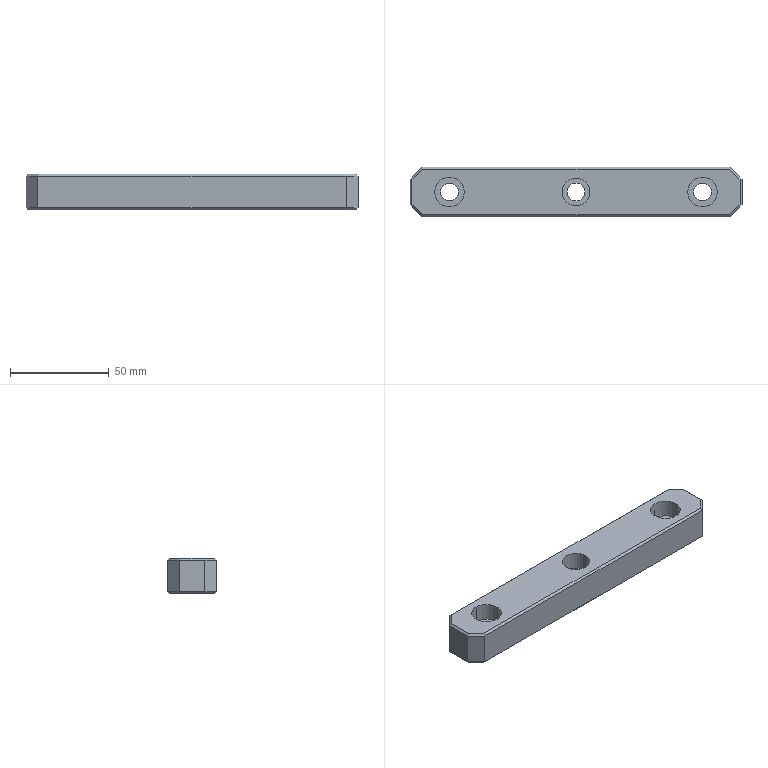Part | Creo | 1 solid | 41 faces | box 168 x 25 x 18 mm | volume 67650 mm3 | plane 29 | cylinder 12 | commonest cylinder face diameters 9 x6 15 x4 14 x2
STEP:
#1=CARTESIAN_POINT('',(281.586,11.495,-63.491));
#2=VERTEX_POINT('',#1);
#3=CARTESIAN_POINT('',(287.,6.081,-63.491));
#4=VERTEX_POINT('',#3);
#5=CARTESIAN_POINT('',(281.586,11.495,-63.491));
#6=DIRECTION('',(0.7071,-0.7071,0.));
#7=VECTOR('',#6,7.657);
#8=LINE('',#5,#7);
#9=EDGE_CURVE('',#2,#4,#8,.T.);
#10=ORIENTED_EDGE('',*,*,#9,.F.);
#11=CARTESIAN_POINT('',(126.414,11.495,-63.491));
#12=VERTEX_POINT('',#11);
#13=CARTESIAN_POINT('',(126.414,11.495,-63.491));
#14=DIRECTION('',(1.,0.,0.));
#15=VECTOR('',#14,155.172);
#16=LINE('',#13,#15);
#17=EDGE_CURVE('',#12,#2,#16,.T.);
#18=ORIENTED_EDGE('',*,*,#17,.F.);
#19=CARTESIAN_POINT('',(121.,6.081,-63.491));
#20=VERTEX_POINT('',#19);
#21=CARTESIAN_POINT('',(121.,6.081,-63.491));
#22=DIRECTION('',(0.7071,0.7071,0.));
#23=VECTOR('',#22,7.657);
#24=LINE('',#21,#23);
#25=EDGE_CURVE('',#20,#12,#24,.T.);
#26=ORIENTED_EDGE('',*,*,#25,.F.);
#27=CARTESIAN_POINT('',(121.,-6.09,-63.491));
#28=VERTEX_POINT('',#27);
#29=CARTESIAN_POINT('',(121.,-6.09,-63.491));
#30=DIRECTION('',(0.,1.,0.));
#31=VECTOR('',#30,12.172);
#32=LINE('',#29,#31);
#33=EDGE_CURVE('',#28,#20,#32,.T.);
#34=ORIENTED_EDGE('',*,*,#33,.F.);
#35=CARTESIAN_POINT('',(126.414,-11.505,-63.491));
#36=VERTEX_POINT('',#35);
#37=CARTESIAN_POINT('',(126.414,-11.505,-63.491));
#38=DIRECTION('',(-0.7071,0.7071,0.));
#39=VECTOR('',#38,7.657);
#40=LINE('',#37,#39);
#41=EDGE_CURVE('',#36,#28,#40,.T.);
#42=ORIENTED_EDGE('',*,*,#41,.F.);
#43=CARTESIAN_POINT('',(281.586,-11.505,-63.491));
#44=VERTEX_POINT('',#43);
#45=CARTESIAN_POINT('',(126.414,-11.505,-63.491));
#46=DIRECTION('',(1.,0.,0.));
#47=VECTOR('',#46,155.172);
#48=LINE('',#45,#47);
#49=EDGE_CURVE('',#36,#44,#48,.T.);
#50=ORIENTED_EDGE('',*,*,#49,.T.);
#51=CARTESIAN_POINT('',(287.,-6.09,-63.491));
#52=VERTEX_POINT('',#51);
#53=CARTESIAN_POINT('',(287.,-6.09,-63.491));
#54=DIRECTION('',(-0.7071,-0.7071,0.));
#55=VECTOR('',#54,7.657);
#56=LINE('',#53,#55);
#57=EDGE_CURVE('',#52,#44,#56,.T.);
#58=ORIENTED_EDGE('',*,*,#57,.F.);
#59=CARTESIAN_POINT('',(287.,6.081,-63.491));
#60=DIRECTION('',(0.,-1.,0.));
#61=VECTOR('',#60,12.172);
#62=LINE('',#59,#61);
#63=EDGE_CURVE('',#4,#52,#62,.T.);
#64=ORIENTED_EDGE('',*,*,#63,.F.);
#65=EDGE_LOOP('',(#10,#18,#26,#34,#42,#50,#58,#64));
#66=FACE_OUTER_BOUND('',#65,.F.);
#67=CARTESIAN_POINT('',(140.,-4.505,-63.491));
#68=VERTEX_POINT('',#67);
#69=CARTESIAN_POINT('',(140.,4.495,-63.491));
#70=VERTEX_POINT('',#69);
#71=CARTESIAN_POINT('',(140.,-0.004699,-63.491));
#72=DIRECTION('',(0.,0.,1.));
#73=DIRECTION('',(0.,-1.,0.));
#74=AXIS2_PLACEMENT_3D('',#71,#72,#73);
#75=CIRCLE('',#74,4.5);
#76=EDGE_CURVE('',#68,#70,#75,.T.);
#77=ORIENTED_EDGE('',*,*,#76,.F.);
#78=CARTESIAN_POINT('',(140.,-0.004699,-63.491));
#79=DIRECTION('',(0.,0.,1.));
#80=DIRECTION('',(0.,1.,0.));
#81=AXIS2_PLACEMENT_3D('',#78,#79,#80);
#82=CIRCLE('',#81,4.5);
#83=EDGE_CURVE('',#70,#68,#82,.T.);
#84=ORIENTED_EDGE('',*,*,#83,.F.);
#85=EDGE_LOOP('',(#77,#84));
#86=FACE_BOUND('',#85,.F.);
#87=CARTESIAN_POINT('',(268.,-4.505,-63.491));
#88=VERTEX_POINT('',#87);
#89=CARTESIAN_POINT('',(268.,4.495,-63.491));
#90=VERTEX_POINT('',#89);
#91=CARTESIAN_POINT('',(268.,-0.004699,-63.491));
#92=DIRECTION('',(0.,0.,1.));
#93=DIRECTION('',(0.,-1.,0.));
#94=AXIS2_PLACEMENT_3D('',#91,#92,#93);
#95=CIRCLE('',#94,4.5);
#96=EDGE_CURVE('',#88,#90,#95,.T.);
#97=ORIENTED_EDGE('',*,*,#96,.F.);
#98=CARTESIAN_POINT('',(268.,-0.004699,-63.491));
#99=DIRECTION('',(0.,0.,1.));
#100=DIRECTION('',(0.,1.,0.));
#101=AXIS2_PLACEMENT_3D('',#98,#99,#100);
#102=CIRCLE('',#101,4.5);
#103=EDGE_CURVE('',#90,#88,#102,.T.);
#104=ORIENTED_EDGE('',*,*,#103,.F.);
#105=EDGE_LOOP('',(#97,#104));
#106=FACE_BOUND('',#105,.F.);
#107=CARTESIAN_POINT('',(208.5,-0.004699,-63.491));
#108=VERTEX_POINT('',#107);
#109=CARTESIAN_POINT('',(199.5,-0.004699,-63.491));
#110=VERTEX_POINT('',#109);
#111=CARTESIAN_POINT('',(204.,-0.004699,-63.491));
#112=DIRECTION('',(0.,0.,1.));
#113=DIRECTION('',(1.,0.,0.));
#114=AXIS2_PLACEMENT_3D('',#111,#112,#113);
#115=CIRCLE('',#114,4.5);
#116=EDGE_CURVE('',#108,#110,#115,.T.);
#117=ORIENTED_EDGE('',*,*,#116,.F.);
#118=CARTESIAN_POINT('',(204.,-0.004699,-63.491));
#119=DIRECTION('',(0.,0.,1.));
#120=DIRECTION('',(-1.,0.,0.));
#121=AXIS2_PLACEMENT_3D('',#118,#119,#120);
#122=CIRCLE('',#121,4.5);
#123=EDGE_CURVE('',#110,#108,#122,.T.);
#124=ORIENTED_EDGE('',*,*,#123,.F.);
#125=EDGE_LOOP('',(#117,#124));
#126=FACE_BOUND('',#125,.F.);
#127=CARTESIAN_POINT('',(270.,-12.505,-63.491));
#128=DIRECTION('',(0.,0.,-1.));
#129=DIRECTION('',(0.,1.,0.));
#130=AXIS2_PLACEMENT_3D('',#127,#128,#129);
#131=PLANE('',#130);
#132=ADVANCED_FACE('',(#66,#86,#106,#126),#131,.T.);
#133=ORIENTED_EDGE('',*,*,#9,.T.);
#134=CARTESIAN_POINT('',(288.,6.495,-62.491));
#135=VERTEX_POINT('',#134);
#136=CARTESIAN_POINT('',(287.,6.081,-63.491));
#137=DIRECTION('',(0.6786,0.2811,0.6786));
#138=VECTOR('',#137,1.474);
#139=LINE('',#136,#138);
#140=EDGE_CURVE('',#4,#135,#139,.T.);
#141=ORIENTED_EDGE('',*,*,#140,.T.);
#142=CARTESIAN_POINT('',(282.,12.495,-62.491));
#143=VERTEX_POINT('',#142);
#144=CARTESIAN_POINT('',(288.,6.495,-62.491));
#145=DIRECTION('',(-0.7071,0.7071,0.));
#146=VECTOR('',#145,8.485);
#147=LINE('',#144,#146);
#148=EDGE_CURVE('',#135,#143,#147,.T.);
#149=ORIENTED_EDGE('',*,*,#148,.T.);
#150=CARTESIAN_POINT('',(281.586,11.495,-63.491));
#151=DIRECTION('',(0.2811,0.6786,0.6786));
#152=VECTOR('',#151,1.474);
#153=LINE('',#150,#152);
#154=EDGE_CURVE('',#2,#143,#153,.T.);
#155=ORIENTED_EDGE('',*,*,#154,.F.);
#156=EDGE_LOOP('',(#133,#141,#149,#155));
#157=FACE_OUTER_BOUND('',#156,.F.);
#158=CARTESIAN_POINT('',(284.646,9.142,-62.991));
#159=DIRECTION('',(0.5,0.5,-0.7071));
#160=DIRECTION('',(0.5,0.5,0.7071));
#161=AXIS2_PLACEMENT_3D('',#158,#159,#160);
#162=PLANE('',#161);
#163=ADVANCED_FACE('',(#157),#162,.T.);
#164=ORIENTED_EDGE('',*,*,#63,.T.);
#165=CARTESIAN_POINT('',(288.,-6.505,-62.491));
#166=VERTEX_POINT('',#165);
#167=CARTESIAN_POINT('',(287.,-6.09,-63.491));
#168=DIRECTION('',(0.6786,-0.2811,0.6786));
#169=VECTOR('',#168,1.474);
#170=LINE('',#167,#169);
#171=EDGE_CURVE('',#52,#166,#170,.T.);
#172=ORIENTED_EDGE('',*,*,#171,.T.);
#173=CARTESIAN_POINT('',(288.,6.495,-62.491));
#174=DIRECTION('',(0.,-1.,0.));
#175=VECTOR('',#174,13.);
#176=LINE('',#173,#175);
#177=EDGE_CURVE('',#135,#166,#176,.T.);
#178=ORIENTED_EDGE('',*,*,#177,.F.);
#179=ORIENTED_EDGE('',*,*,#140,.F.);
#180=EDGE_LOOP('',(#164,#172,#178,#179));
#181=FACE_OUTER_BOUND('',#180,.F.);
#182=CARTESIAN_POINT('',(287.5,-0.004699,-62.991));
#183=DIRECTION('',(0.7071,0.,-0.7071));
#184=DIRECTION('',(-0.7071,0.,-0.7071));
#185=AXIS2_PLACEMENT_3D('',#182,#183,#184);
#186=PLANE('',#185);
#187=ADVANCED_FACE('',(#181),#186,.T.);
#188=ORIENTED_EDGE('',*,*,#57,.T.);
#189=CARTESIAN_POINT('',(282.,-12.505,-62.491));
#190=VERTEX_POINT('',#189);
#191=CARTESIAN_POINT('',(281.586,-11.505,-63.491));
#192=DIRECTION('',(0.2811,-0.6786,0.6786));
#193=VECTOR('',#192,1.474);
#194=LINE('',#191,#193);
#195=EDGE_CURVE('',#44,#190,#194,.T.);
#196=ORIENTED_EDGE('',*,*,#195,.T.);
#197=CARTESIAN_POINT('',(282.,-12.505,-62.491));
#198=DIRECTION('',(0.7071,0.7071,0.));
#199=VECTOR('',#198,8.485);
#200=LINE('',#197,#199);
#201=EDGE_CURVE('',#190,#166,#200,.T.);
#202=ORIENTED_EDGE('',*,*,#201,.T.);
#203=ORIENTED_EDGE('',*,*,#171,.F.);
#204=EDGE_LOOP('',(#188,#196,#202,#203));
#205=FACE_OUTER_BOUND('',#204,.F.);
#206=CARTESIAN_POINT('',(284.646,-9.151,-62.991));
#207=DIRECTION('',(0.5,-0.5,-0.7071));
#208=DIRECTION('',(0.5,-0.5,0.7071));
#209=AXIS2_PLACEMENT_3D('',#206,#207,#208);
#210=PLANE('',#209);
#211=ADVANCED_FACE('',(#205),#210,.T.);
#212=CARTESIAN_POINT('',(126.,-12.505,-62.491));
#213=VERTEX_POINT('',#212);
#214=CARTESIAN_POINT('',(126.,-12.505,-62.491));
#215=DIRECTION('',(0.2811,0.6786,-0.6786));
#216=VECTOR('',#215,1.474);
#217=LINE('',#214,#216);
#218=EDGE_CURVE('',#213,#36,#217,.T.);
#219=ORIENTED_EDGE('',*,*,#218,.F.);
#220=CARTESIAN_POINT('',(126.,-12.505,-62.491));
#221=DIRECTION('',(1.,0.,0.));
#222=VECTOR('',#221,156.);
#223=LINE('',#220,#222);
#224=EDGE_CURVE('',#213,#190,#223,.T.);
#225=ORIENTED_EDGE('',*,*,#224,.T.);
#226=ORIENTED_EDGE('',*,*,#195,.F.);
#227=ORIENTED_EDGE('',*,*,#49,.F.);
#228=EDGE_LOOP('',(#219,#225,#226,#227));
#229=FACE_OUTER_BOUND('',#228,.F.);
#230=CARTESIAN_POINT('',(174.,-12.005,-62.991));
#231=DIRECTION('',(0.,-0.7071,-0.7071));
#232=DIRECTION('',(0.,-0.7071,0.7071));
#233=AXIS2_PLACEMENT_3D('',#230,#231,#232);
#234=PLANE('',#233);
#235=ADVANCED_FACE('',(#229),#234,.T.);
#236=CARTESIAN_POINT('',(120.,-6.505,-62.491));
#237=VERTEX_POINT('',#236);
#238=CARTESIAN_POINT('',(120.,-6.505,-62.491));
#239=DIRECTION('',(0.7071,-0.7071,0.));
#240=VECTOR('',#239,8.485);
#241=LINE('',#238,#240);
#242=EDGE_CURVE('',#237,#213,#241,.T.);
#243=ORIENTED_EDGE('',*,*,#242,.T.);
#244=ORIENTED_EDGE('',*,*,#218,.T.);
#245=ORIENTED_EDGE('',*,*,#41,.T.);
#246=CARTESIAN_POINT('',(121.,-6.09,-63.491));
#247=DIRECTION('',(-0.6786,-0.2811,0.6786));
#248=VECTOR('',#247,1.474);
#249=LINE('',#246,#248);
#250=EDGE_CURVE('',#28,#237,#249,.T.);
#251=ORIENTED_EDGE('',*,*,#250,.T.);
#252=EDGE_LOOP('',(#243,#244,#245,#251));
#253=FACE_OUTER_BOUND('',#252,.F.);
#254=CARTESIAN_POINT('',(123.354,-9.151,-62.991));
#255=DIRECTION('',(-0.5,-0.5,-0.7071));
#256=DIRECTION('',(-0.5,-0.5,0.7071));
#257=AXIS2_PLACEMENT_3D('',#254,#255,#256);
#258=PLANE('',#257);
#259=ADVANCED_FACE('',(#253),#258,.T.);
#260=CARTESIAN_POINT('',(126.,-12.505,-46.491));
#261=VERTEX_POINT('',#260);
#262=CARTESIAN_POINT('',(126.,-12.505,-46.491));
#263=DIRECTION('',(0.,0.,-1.));
#264=VECTOR('',#263,16.);
#265=LINE('',#262,#264);
#266=EDGE_CURVE('',#261,#213,#265,.T.);
#267=ORIENTED_EDGE('',*,*,#266,.T.);
#268=ORIENTED_EDGE('',*,*,#242,.F.);
#269=CARTESIAN_POINT('',(120.,-6.505,-46.491));
#270=VERTEX_POINT('',#269);
#271=CARTESIAN_POINT('',(120.,-6.505,-46.491));
#272=DIRECTION('',(0.,0.,-1.));
#273=VECTOR('',#272,16.);
#274=LINE('',#271,#273);
#275=EDGE_CURVE('',#270,#237,#274,.T.);
#276=ORIENTED_EDGE('',*,*,#275,.F.);
#277=CARTESIAN_POINT('',(120.,-6.505,-46.491));
#278=DIRECTION('',(0.7071,-0.7071,0.));
#279=VECTOR('',#278,8.485);
#280=LINE('',#277,#279);
#281=EDGE_CURVE('',#270,#261,#280,.T.);
#282=ORIENTED_EDGE('',*,*,#281,.T.);
#283=EDGE_LOOP('',(#267,#268,#276,#282));
#284=FACE_OUTER_BOUND('',#283,.F.);
#285=CARTESIAN_POINT('',(123.,-9.505,-54.491));
#286=DIRECTION('',(-0.7071,-0.7071,0.));
#287=DIRECTION('',(0.,0.,1.));
#288=AXIS2_PLACEMENT_3D('',#285,#286,#287);
#289=PLANE('',#288);
#290=ADVANCED_FACE('',(#284),#289,.T.);
#291=CARTESIAN_POINT('',(282.,-12.505,-46.491));
#292=VERTEX_POINT('',#291);
#293=CARTESIAN_POINT('',(282.,-12.505,-62.491));
#294=DIRECTION('',(0.,0.,1.));
#295=VECTOR('',#294,16.);
#296=LINE('',#293,#295);
#297=EDGE_CURVE('',#190,#292,#296,.T.);
#298=ORIENTED_EDGE('',*,*,#297,.F.);
#299=ORIENTED_EDGE('',*,*,#224,.F.);
#300=ORIENTED_EDGE('',*,*,#266,.F.);
#301=CARTESIAN_POINT('',(126.,-12.505,-46.491));
#302=DIRECTION('',(1.,0.,0.));
#303=VECTOR('',#302,156.);
#304=LINE('',#301,#303);
#305=EDGE_CURVE('',#261,#292,#304,.T.);
#306=ORIENTED_EDGE('',*,*,#305,.T.);
#307=EDGE_LOOP('',(#298,#299,#300,#306));
#308=FACE_OUTER_BOUND('',#307,.F.);
#309=CARTESIAN_POINT('',(270.,-12.505,-45.491));
#310=DIRECTION('',(0.,-1.,0.));
#311=DIRECTION('',(0.,0.,-1.));
#312=AXIS2_PLACEMENT_3D('',#309,#310,#311);
#313=PLANE('',#312);
#314=ADVANCED_FACE('',(#308),#313,.T.);
#315=CARTESIAN_POINT('',(288.,-6.505,-46.491));
#316=VERTEX_POINT('',#315);
#317=CARTESIAN_POINT('',(288.,-6.505,-62.491));
#318=DIRECTION('',(0.,0.,1.));
#319=VECTOR('',#318,16.);
#320=LINE('',#317,#319);
#321=EDGE_CURVE('',#166,#316,#320,.T.);
#322=ORIENTED_EDGE('',*,*,#321,.F.);
#323=ORIENTED_EDGE('',*,*,#201,.F.);
#324=ORIENTED_EDGE('',*,*,#297,.T.);
#325=CARTESIAN_POINT('',(282.,-12.505,-46.491));
#326=DIRECTION('',(0.7071,0.7071,0.));
#327=VECTOR('',#326,8.485);
#328=LINE('',#325,#327);
#329=EDGE_CURVE('',#292,#316,#328,.T.);
#330=ORIENTED_EDGE('',*,*,#329,.T.);
#331=EDGE_LOOP('',(#322,#323,#324,#330));
#332=FACE_OUTER_BOUND('',#331,.F.);
#333=CARTESIAN_POINT('',(285.,-9.505,-54.491));
#334=DIRECTION('',(0.7071,-0.7071,0.));
#335=DIRECTION('',(0.,0.,1.));
#336=AXIS2_PLACEMENT_3D('',#333,#334,#335);
#337=PLANE('',#336);
#338=ADVANCED_FACE('',(#332),#337,.T.);
#339=CARTESIAN_POINT('',(288.,6.495,-46.491));
#340=VERTEX_POINT('',#339);
#341=CARTESIAN_POINT('',(288.,6.495,-46.491));
#342=DIRECTION('',(0.,0.,-1.));
#343=VECTOR('',#342,16.);
#344=LINE('',#341,#343);
#345=EDGE_CURVE('',#340,#135,#344,.T.);
#346=ORIENTED_EDGE('',*,*,#345,.T.);
#347=ORIENTED_EDGE('',*,*,#177,.T.);
#348=ORIENTED_EDGE('',*,*,#321,.T.);
#349=CARTESIAN_POINT('',(288.,-6.505,-46.491));
#350=DIRECTION('',(0.,1.,0.));
#351=VECTOR('',#350,13.);
#352=LINE('',#349,#351);
#353=EDGE_CURVE('',#316,#340,#352,.T.);
#354=ORIENTED_EDGE('',*,*,#353,.T.);
#355=EDGE_LOOP('',(#346,#347,#348,#354));
#356=FACE_OUTER_BOUND('',#355,.F.);
#357=CARTESIAN_POINT('',(288.,-0.004699,-53.491));
#358=DIRECTION('',(1.,0.,0.));
#359=DIRECTION('',(0.,1.,0.));
#360=AXIS2_PLACEMENT_3D('',#357,#358,#359);
#361=PLANE('',#360);
#362=ADVANCED_FACE('',(#356),#361,.T.);
#363=CARTESIAN_POINT('',(282.,12.495,-46.491));
#364=VERTEX_POINT('',#363);
#365=CARTESIAN_POINT('',(282.,12.495,-46.491));
#366=DIRECTION('',(0.,0.,-1.));
#367=VECTOR('',#366,16.);
#368=LINE('',#365,#367);
#369=EDGE_CURVE('',#364,#143,#368,.T.);
#370=ORIENTED_EDGE('',*,*,#369,.T.);
#371=ORIENTED_EDGE('',*,*,#148,.F.);
#372=ORIENTED_EDGE('',*,*,#345,.F.);
#373=CARTESIAN_POINT('',(288.,6.495,-46.491));
#374=DIRECTION('',(-0.7071,0.7071,0.));
#375=VECTOR('',#374,8.485);
#376=LINE('',#373,#375);
#377=EDGE_CURVE('',#340,#364,#376,.T.);
#378=ORIENTED_EDGE('',*,*,#377,.T.);
#379=EDGE_LOOP('',(#370,#371,#372,#378));
#380=FACE_OUTER_BOUND('',#379,.F.);
#381=CARTESIAN_POINT('',(285.,9.495,-54.491));
#382=DIRECTION('',(0.7071,0.7071,0.));
#383=DIRECTION('',(0.,0.,1.));
#384=AXIS2_PLACEMENT_3D('',#381,#382,#383);
#385=PLANE('',#384);
#386=ADVANCED_FACE('',(#380),#385,.T.);
#387=CARTESIAN_POINT('',(126.,12.495,-62.491));
#388=VERTEX_POINT('',#387);
#389=CARTESIAN_POINT('',(126.,12.495,-46.491));
#390=VERTEX_POINT('',#389);
#391=CARTESIAN_POINT('',(126.,12.495,-62.491));
#392=DIRECTION('',(0.,0.,1.));
#393=VECTOR('',#392,16.);
#394=LINE('',#391,#393);
#395=EDGE_CURVE('',#388,#390,#394,.T.);
#396=ORIENTED_EDGE('',*,*,#395,.F.);
#397=CARTESIAN_POINT('',(126.,12.495,-62.491));
#398=DIRECTION('',(1.,0.,0.));
#399=VECTOR('',#398,156.);
#400=LINE('',#397,#399);
#401=EDGE_CURVE('',#388,#143,#400,.T.);
#402=ORIENTED_EDGE('',*,*,#401,.T.);
#403=ORIENTED_EDGE('',*,*,#369,.F.);
#404=CARTESIAN_POINT('',(126.,12.495,-46.491));
#405=DIRECTION('',(1.,0.,0.));
#406=VECTOR('',#405,156.);
#407=LINE('',#404,#406);
#408=EDGE_CURVE('',#390,#364,#407,.T.);
#409=ORIENTED_EDGE('',*,*,#408,.F.);
#410=EDGE_LOOP('',(#396,#402,#403,#409));
#411=FACE_OUTER_BOUND('',#410,.F.);
#412=CARTESIAN_POINT('',(270.,12.495,-63.491));
#413=DIRECTION('',(0.,1.,0.));
#414=DIRECTION('',(0.,0.,1.));
#415=AXIS2_PLACEMENT_3D('',#412,#413,#414);
#416=PLANE('',#415);
#417=ADVANCED_FACE('',(#411),#416,.T.);
#418=CARTESIAN_POINT('',(120.,6.495,-62.491));
#419=VERTEX_POINT('',#418);
#420=CARTESIAN_POINT('',(120.,6.495,-46.491));
#421=VERTEX_POINT('',#420);
#422=CARTESIAN_POINT('',(120.,6.495,-62.491));
#423=DIRECTION('',(0.,0.,1.));
#424=VECTOR('',#423,16.);
#425=LINE('',#422,#424);
#426=EDGE_CURVE('',#419,#421,#425,.T.);
#427=ORIENTED_EDGE('',*,*,#426,.F.);
#428=CARTESIAN_POINT('',(126.,12.495,-62.491));
#429=DIRECTION('',(-0.7071,-0.7071,0.));
#430=VECTOR('',#429,8.485);
#431=LINE('',#428,#430);
#432=EDGE_CURVE('',#388,#419,#431,.T.);
#433=ORIENTED_EDGE('',*,*,#432,.F.);
#434=ORIENTED_EDGE('',*,*,#395,.T.);
#435=CARTESIAN_POINT('',(126.,12.495,-46.491));
#436=DIRECTION('',(-0.7071,-0.7071,0.));
#437=VECTOR('',#436,8.485);
#438=LINE('',#435,#437);
#439=EDGE_CURVE('',#390,#421,#438,.T.);
#440=ORIENTED_EDGE('',*,*,#439,.T.);
#441=EDGE_LOOP('',(#427,#433,#434,#440));
#442=FACE_OUTER_BOUND('',#441,.F.);
#443=CARTESIAN_POINT('',(123.,9.495,-54.491));
#444=DIRECTION('',(-0.7071,0.7071,0.));
#445=DIRECTION('',(0.,0.,1.));
#446=AXIS2_PLACEMENT_3D('',#443,#444,#445);
#447=PLANE('',#446);
#448=ADVANCED_FACE('',(#442),#447,.T.);
#449=ORIENTED_EDGE('',*,*,#275,.T.);
#450=CARTESIAN_POINT('',(120.,-6.505,-62.491));
#451=DIRECTION('',(0.,1.,0.));
#452=VECTOR('',#451,13.);
#453=LINE('',#450,#452);
#454=EDGE_CURVE('',#237,#419,#453,.T.);
#455=ORIENTED_EDGE('',*,*,#454,.T.);
#456=ORIENTED_EDGE('',*,*,#426,.T.);
#457=CARTESIAN_POINT('',(120.,6.495,-46.491));
#458=DIRECTION('',(0.,-1.,0.));
#459=VECTOR('',#458,13.);
#460=LINE('',#457,#459);
#461=EDGE_CURVE('',#421,#270,#460,.T.);
#462=ORIENTED_EDGE('',*,*,#461,.T.);
#463=EDGE_LOOP('',(#449,#455,#456,#462));
#464=FACE_OUTER_BOUND('',#463,.F.);
#465=CARTESIAN_POINT('',(120.,-0.004699,-53.491));
#466=DIRECTION('',(1.,0.,0.));
#467=DIRECTION('',(0.,1.,0.));
#468=AXIS2_PLACEMENT_3D('',#465,#466,#467);
#469=PLANE('',#468);
#470=ADVANCED_FACE('',(#464),#469,.F.);
#471=ORIENTED_EDGE('',*,*,#33,.T.);
#472=CARTESIAN_POINT('',(121.,6.081,-63.491));
#473=DIRECTION('',(-0.6786,0.2811,0.6786));
#474=VECTOR('',#473,1.474);
#475=LINE('',#472,#474);
#476=EDGE_CURVE('',#20,#419,#475,.T.);
#477=ORIENTED_EDGE('',*,*,#476,.T.);
#478=ORIENTED_EDGE('',*,*,#454,.F.);
#479=ORIENTED_EDGE('',*,*,#250,.F.);
#480=EDGE_LOOP('',(#471,#477,#478,#479));
#481=FACE_OUTER_BOUND('',#480,.F.);
#482=CARTESIAN_POINT('',(120.5,-0.004699,-62.991));
#483=DIRECTION('',(-0.7071,0.,-0.7071));
#484=DIRECTION('',(0.7071,0.,-0.7071));
#485=AXIS2_PLACEMENT_3D('',#482,#483,#484);
#486=PLANE('',#485);
#487=ADVANCED_FACE('',(#481),#486,.T.);
#488=ORIENTED_EDGE('',*,*,#25,.T.);
#489=CARTESIAN_POINT('',(126.414,11.495,-63.491));
#490=DIRECTION('',(-0.2811,0.6786,0.6786));
#491=VECTOR('',#490,1.474);
#492=LINE('',#489,#491);
#493=EDGE_CURVE('',#12,#388,#492,.T.);
#494=ORIENTED_EDGE('',*,*,#493,.T.);
#495=ORIENTED_EDGE('',*,*,#432,.T.);
#496=ORIENTED_EDGE('',*,*,#476,.F.);
#497=EDGE_LOOP('',(#488,#494,#495,#496));
#498=FACE_OUTER_BOUND('',#497,.F.);
#499=CARTESIAN_POINT('',(123.354,9.142,-62.991));
#500=DIRECTION('',(-0.5,0.5,-0.7071));
#501=DIRECTION('',(-0.5,0.5,0.7071));
#502=AXIS2_PLACEMENT_3D('',#499,#500,#501);
#503=PLANE('',#502);
#504=ADVANCED_FACE('',(#498),#503,.T.);
#505=ORIENTED_EDGE('',*,*,#493,.F.);
#506=ORIENTED_EDGE('',*,*,#17,.T.);
#507=ORIENTED_EDGE('',*,*,#154,.T.);
#508=ORIENTED_EDGE('',*,*,#401,.F.);
#509=EDGE_LOOP('',(#505,#506,#507,#508));
#510=FACE_OUTER_BOUND('',#509,.F.);
#511=CARTESIAN_POINT('',(174.,11.995,-62.991));
#512=DIRECTION('',(0.,0.7071,-0.7071));
#513=DIRECTION('',(0.,-0.7071,-0.7071));
#514=AXIS2_PLACEMENT_3D('',#511,#512,#513);
#515=PLANE('',#514);
#516=ADVANCED_FACE('',(#510),#515,.T.);
#517=CARTESIAN_POINT('',(121.,6.081,-45.491));
#518=VERTEX_POINT('',#517);
#519=CARTESIAN_POINT('',(121.,-6.09,-45.491));
#520=VERTEX_POINT('',#519);
#521=CARTESIAN_POINT('',(121.,6.081,-45.491));
#522=DIRECTION('',(0.,-1.,0.));
#523=VECTOR('',#522,12.172);
#524=LINE('',#521,#523);
#525=EDGE_CURVE('',#518,#520,#524,.T.);
#526=ORIENTED_EDGE('',*,*,#525,.T.);
#527=CARTESIAN_POINT('',(121.,-6.09,-45.491));
#528=DIRECTION('',(-0.6786,-0.2811,-0.6786));
#529=VECTOR('',#528,1.474);
#530=LINE('',#527,#529);
#531=EDGE_CURVE('',#520,#270,#530,.T.);
#532=ORIENTED_EDGE('',*,*,#531,.T.);
#533=ORIENTED_EDGE('',*,*,#461,.F.);
#534=CARTESIAN_POINT('',(121.,6.081,-45.491));
#535=DIRECTION('',(-0.6786,0.2811,-0.6786));
#536=VECTOR('',#535,1.474);
#537=LINE('',#534,#536);
#538=EDGE_CURVE('',#518,#421,#537,.T.);
#539=ORIENTED_EDGE('',*,*,#538,.F.);
#540=EDGE_LOOP('',(#526,#532,#533,#539));
#541=FACE_OUTER_BOUND('',#540,.F.);
#542=CARTESIAN_POINT('',(120.5,-0.004699,-45.991));
#543=DIRECTION('',(-0.7071,0.,0.7071));
#544=DIRECTION('',(0.,-1.,0.));
#545=AXIS2_PLACEMENT_3D('',#542,#543,#544);
#546=PLANE('',#545);
#547=ADVANCED_FACE('',(#541),#546,.T.);
#548=CARTESIAN_POINT('',(287.,-6.09,-45.491));
#549=VERTEX_POINT('',#548);
#550=CARTESIAN_POINT('',(281.586,-11.505,-45.491));
#551=VERTEX_POINT('',#550);
#552=CARTESIAN_POINT('',(287.,-6.09,-45.491));
#553=DIRECTION('',(-0.7071,-0.7071,0.));
#554=VECTOR('',#553,7.657);
#555=LINE('',#552,#554);
#556=EDGE_CURVE('',#549,#551,#555,.T.);
#557=ORIENTED_EDGE('',*,*,#556,.T.);
#558=CARTESIAN_POINT('',(126.414,-11.505,-45.491));
#559=VERTEX_POINT('',#558);
#560=CARTESIAN_POINT('',(126.414,-11.505,-45.491));
#561=DIRECTION('',(1.,0.,0.));
#562=VECTOR('',#561,155.172);
#563=LINE('',#560,#562);
#564=EDGE_CURVE('',#559,#551,#563,.T.);
#565=ORIENTED_EDGE('',*,*,#564,.F.);
#566=CARTESIAN_POINT('',(126.414,-11.505,-45.491));
#567=DIRECTION('',(-0.7071,0.7071,0.));
#568=VECTOR('',#567,7.657);
#569=LINE('',#566,#568);
#570=EDGE_CURVE('',#559,#520,#569,.T.);
#571=ORIENTED_EDGE('',*,*,#570,.T.);
#572=ORIENTED_EDGE('',*,*,#525,.F.);
#573=CARTESIAN_POINT('',(126.414,11.495,-45.491));
#574=VERTEX_POINT('',#573);
#575=CARTESIAN_POINT('',(121.,6.081,-45.491));
#576=DIRECTION('',(0.7071,0.7071,0.));
#577=VECTOR('',#576,7.657);
#578=LINE('',#575,#577);
#579=EDGE_CURVE('',#518,#574,#578,.T.);
#580=ORIENTED_EDGE('',*,*,#579,.T.);
#581=CARTESIAN_POINT('',(281.586,11.495,-45.491));
#582=VERTEX_POINT('',#581);
#583=CARTESIAN_POINT('',(126.414,11.495,-45.491));
#584=DIRECTION('',(1.,0.,0.));
#585=VECTOR('',#584,155.172);
#586=LINE('',#583,#585);
#587=EDGE_CURVE('',#574,#582,#586,.T.);
#588=ORIENTED_EDGE('',*,*,#587,.T.);
#589=CARTESIAN_POINT('',(287.,6.081,-45.491));
#590=VERTEX_POINT('',#589);
#591=CARTESIAN_POINT('',(281.586,11.495,-45.491));
#592=DIRECTION('',(0.7071,-0.7071,0.));
#593=VECTOR('',#592,7.657);
#594=LINE('',#591,#593);
#595=EDGE_CURVE('',#582,#590,#594,.T.);
#596=ORIENTED_EDGE('',*,*,#595,.T.);
#597=CARTESIAN_POINT('',(287.,-6.09,-45.491));
#598=DIRECTION('',(0.,1.,0.));
#599=VECTOR('',#598,12.172);
#600=LINE('',#597,#599);
#601=EDGE_CURVE('',#549,#590,#600,.T.);
#602=ORIENTED_EDGE('',*,*,#601,.F.);
#603=EDGE_LOOP('',(#557,#565,#571,#572,#580,#588,#596,#602));
#604=FACE_OUTER_BOUND('',#603,.F.);
#605=CARTESIAN_POINT('',(268.,-7.505,-45.491));
#606=VERTEX_POINT('',#605);
#607=CARTESIAN_POINT('',(268.,7.495,-45.491));
#608=VERTEX_POINT('',#607);
#609=CARTESIAN_POINT('',(268.,-0.004699,-45.491));
#610=DIRECTION('',(0.,0.,-1.));
#611=DIRECTION('',(0.,-1.,0.));
#612=AXIS2_PLACEMENT_3D('',#609,#610,#611);
#613=CIRCLE('',#612,7.5);
#614=EDGE_CURVE('',#606,#608,#613,.T.);
#615=ORIENTED_EDGE('',*,*,#614,.F.);
#616=CARTESIAN_POINT('',(268.,-0.004699,-45.491));
#617=DIRECTION('',(0.,0.,-1.));
#618=DIRECTION('',(0.,1.,0.));
#619=AXIS2_PLACEMENT_3D('',#616,#617,#618);
#620=CIRCLE('',#619,7.5);
#621=EDGE_CURVE('',#608,#606,#620,.T.);
#622=ORIENTED_EDGE('',*,*,#621,.F.);
#623=EDGE_LOOP('',(#615,#622));
#624=FACE_BOUND('',#623,.F.);
#625=CARTESIAN_POINT('',(140.,-7.505,-45.491));
#626=VERTEX_POINT('',#625);
#627=CARTESIAN_POINT('',(140.,7.495,-45.491));
#628=VERTEX_POINT('',#627);
#629=CARTESIAN_POINT('',(140.,-0.004699,-45.491));
#630=DIRECTION('',(0.,0.,-1.));
#631=DIRECTION('',(0.,-1.,0.));
#632=AXIS2_PLACEMENT_3D('',#629,#630,#631);
#633=CIRCLE('',#632,7.5);
#634=EDGE_CURVE('',#626,#628,#633,.T.);
#635=ORIENTED_EDGE('',*,*,#634,.F.);
#636=CARTESIAN_POINT('',(140.,-0.004699,-45.491));
#637=DIRECTION('',(0.,0.,-1.));
#638=DIRECTION('',(0.,1.,0.));
#639=AXIS2_PLACEMENT_3D('',#636,#637,#638);
#640=CIRCLE('',#639,7.5);
#641=EDGE_CURVE('',#628,#626,#640,.T.);
#642=ORIENTED_EDGE('',*,*,#641,.F.);
#643=EDGE_LOOP('',(#635,#642));
#644=FACE_BOUND('',#643,.F.);
#645=CARTESIAN_POINT('',(211.,-0.004699,-45.491));
#646=VERTEX_POINT('',#645);
#647=CARTESIAN_POINT('',(197.,-0.004699,-45.491));
#648=VERTEX_POINT('',#647);
#649=CARTESIAN_POINT('',(204.,-0.004699,-45.491));
#650=DIRECTION('',(0.,0.,-1.));
#651=DIRECTION('',(1.,0.,0.));
#652=AXIS2_PLACEMENT_3D('',#649,#650,#651);
#653=CIRCLE('',#652,7.);
#654=EDGE_CURVE('',#646,#648,#653,.T.);
#655=ORIENTED_EDGE('',*,*,#654,.F.);
#656=CARTESIAN_POINT('',(204.,-0.004699,-45.491));
#657=DIRECTION('',(0.,0.,-1.));
#658=DIRECTION('',(-1.,0.,0.));
#659=AXIS2_PLACEMENT_3D('',#656,#657,#658);
#660=CIRCLE('',#659,7.);
#661=EDGE_CURVE('',#648,#646,#660,.T.);
#662=ORIENTED_EDGE('',*,*,#661,.F.);
#663=EDGE_LOOP('',(#655,#662));
#664=FACE_BOUND('',#663,.F.);
#665=CARTESIAN_POINT('',(270.,12.495,-45.491));
#666=DIRECTION('',(0.,0.,1.));
#667=DIRECTION('',(0.,-1.,0.));
#668=AXIS2_PLACEMENT_3D('',#665,#666,#667);
#669=PLANE('',#668);
#670=ADVANCED_FACE('',(#604,#624,#644,#664),#669,.T.);
#671=CARTESIAN_POINT('',(197.,-0.004699,-54.491));
#672=VERTEX_POINT('',#671);
#673=CARTESIAN_POINT('',(211.,-0.004699,-54.491));
#674=VERTEX_POINT('',#673);
#675=CARTESIAN_POINT('',(204.,-0.004699,-54.491));
#676=DIRECTION('',(0.,0.,1.));
#677=DIRECTION('',(-1.,0.,0.));
#678=AXIS2_PLACEMENT_3D('',#675,#676,#677);
#679=CIRCLE('',#678,7.);
#680=EDGE_CURVE('',#672,#674,#679,.T.);
#681=ORIENTED_EDGE('',*,*,#680,.T.);
#682=CARTESIAN_POINT('',(211.,-0.004699,-54.491));
#683=DIRECTION('',(0.,0.,1.));
#684=VECTOR('',#683,9.);
#685=LINE('',#682,#684);
#686=EDGE_CURVE('',#674,#646,#685,.T.);
#687=ORIENTED_EDGE('',*,*,#686,.T.);
#688=ORIENTED_EDGE('',*,*,#654,.T.);
#689=CARTESIAN_POINT('',(197.,-0.004699,-54.491));
#690=DIRECTION('',(0.,0.,1.));
#691=VECTOR('',#690,9.);
#692=LINE('',#689,#691);
#693=EDGE_CURVE('',#672,#648,#692,.T.);
#694=ORIENTED_EDGE('',*,*,#693,.F.);
#695=EDGE_LOOP('',(#681,#687,#688,#694));
#696=FACE_OUTER_BOUND('',#695,.F.);
#697=CARTESIAN_POINT('',(204.,-0.004699,-45.491));
#698=DIRECTION('',(0.,0.,1.));
#699=DIRECTION('',(1.,0.,0.));
#700=AXIS2_PLACEMENT_3D('',#697,#698,#699);
#701=CYLINDRICAL_SURFACE('',#700,7.);
#702=ADVANCED_FACE('',(#696),#701,.F.);
#703=CARTESIAN_POINT('',(204.,-0.004699,-54.491));
#704=DIRECTION('',(0.,0.,1.));
#705=DIRECTION('',(1.,0.,0.));
#706=AXIS2_PLACEMENT_3D('',#703,#704,#705);
#707=CIRCLE('',#706,7.);
#708=EDGE_CURVE('',#674,#672,#707,.T.);
#709=ORIENTED_EDGE('',*,*,#708,.F.);
#710=ORIENTED_EDGE('',*,*,#680,.F.);
#711=EDGE_LOOP('',(#709,#710));
#712=FACE_OUTER_BOUND('',#711,.F.);
#713=CARTESIAN_POINT('',(208.5,-0.004699,-54.491));
#714=VERTEX_POINT('',#713);
#715=CARTESIAN_POINT('',(199.5,-0.004699,-54.491));
#716=VERTEX_POINT('',#715);
#717=CARTESIAN_POINT('',(204.,-0.004699,-54.491));
#718=DIRECTION('',(0.,0.,-1.));
#719=DIRECTION('',(1.,0.,0.));
#720=AXIS2_PLACEMENT_3D('',#717,#718,#719);
#721=CIRCLE('',#720,4.5);
#722=EDGE_CURVE('',#714,#716,#721,.T.);
#723=ORIENTED_EDGE('',*,*,#722,.F.);
#724=CARTESIAN_POINT('',(204.,-0.004699,-54.491));
#725=DIRECTION('',(0.,0.,-1.));
#726=DIRECTION('',(-1.,0.,0.));
#727=AXIS2_PLACEMENT_3D('',#724,#725,#726);
#728=CIRCLE('',#727,4.5);
#729=EDGE_CURVE('',#716,#714,#728,.T.);
#730=ORIENTED_EDGE('',*,*,#729,.F.);
#731=EDGE_LOOP('',(#723,#730));
#732=FACE_BOUND('',#731,.F.);
#733=CARTESIAN_POINT('',(204.,6.995,-54.491));
#734=DIRECTION('',(0.,0.,-1.));
#735=DIRECTION('',(-1.,0.,0.));
#736=AXIS2_PLACEMENT_3D('',#733,#734,#735);
#737=PLANE('',#736);
#738=ADVANCED_FACE('',(#712,#732),#737,.F.);
#739=ORIENTED_EDGE('',*,*,#123,.T.);
#740=CARTESIAN_POINT('',(208.5,-0.004699,-63.491));
#741=DIRECTION('',(0.,0.,1.));
#742=VECTOR('',#741,9.);
#743=LINE('',#740,#742);
#744=EDGE_CURVE('',#108,#714,#743,.T.);
#745=ORIENTED_EDGE('',*,*,#744,.T.);
#746=ORIENTED_EDGE('',*,*,#722,.T.);
#747=CARTESIAN_POINT('',(199.5,-0.004699,-63.491));
#748=DIRECTION('',(0.,0.,1.));
#749=VECTOR('',#748,9.);
#750=LINE('',#747,#749);
#751=EDGE_CURVE('',#110,#716,#750,.T.);
#752=ORIENTED_EDGE('',*,*,#751,.F.);
#753=EDGE_LOOP('',(#739,#745,#746,#752));
#754=FACE_OUTER_BOUND('',#753,.F.);
#755=CARTESIAN_POINT('',(204.,-0.004699,-45.491));
#756=DIRECTION('',(0.,0.,1.));
#757=DIRECTION('',(1.,0.,0.));
#758=AXIS2_PLACEMENT_3D('',#755,#756,#757);
#759=CYLINDRICAL_SURFACE('',#758,4.5);
#760=ADVANCED_FACE('',(#754),#759,.F.);
#761=ORIENTED_EDGE('',*,*,#116,.T.);
#762=ORIENTED_EDGE('',*,*,#751,.T.);
#763=ORIENTED_EDGE('',*,*,#729,.T.);
#764=ORIENTED_EDGE('',*,*,#744,.F.);
#765=EDGE_LOOP('',(#761,#762,#763,#764));
#766=FACE_OUTER_BOUND('',#765,.F.);
#767=CARTESIAN_POINT('',(204.,-0.004699,-45.491));
#768=DIRECTION('',(0.,0.,1.));
#769=DIRECTION('',(1.,0.,0.));
#770=AXIS2_PLACEMENT_3D('',#767,#768,#769);
#771=CYLINDRICAL_SURFACE('',#770,4.5);
#772=ADVANCED_FACE('',(#766),#771,.F.);
#773=ORIENTED_EDGE('',*,*,#708,.T.);
#774=ORIENTED_EDGE('',*,*,#693,.T.);
#775=ORIENTED_EDGE('',*,*,#661,.T.);
#776=ORIENTED_EDGE('',*,*,#686,.F.);
#777=EDGE_LOOP('',(#773,#774,#775,#776));
#778=FACE_OUTER_BOUND('',#777,.F.);
#779=CARTESIAN_POINT('',(204.,-0.004699,-45.491));
#780=DIRECTION('',(0.,0.,1.));
#781=DIRECTION('',(1.,0.,0.));
#782=AXIS2_PLACEMENT_3D('',#779,#780,#781);
#783=CYLINDRICAL_SURFACE('',#782,7.);
#784=ADVANCED_FACE('',(#778),#783,.F.);
#785=CARTESIAN_POINT('',(268.,-7.505,-54.491));
#786=VERTEX_POINT('',#785);
#787=CARTESIAN_POINT('',(268.,-7.505,-54.491));
#788=DIRECTION('',(0.,0.,1.));
#789=VECTOR('',#788,9.);
#790=LINE('',#787,#789);
#791=EDGE_CURVE('',#786,#606,#790,.T.);
#792=ORIENTED_EDGE('',*,*,#791,.T.);
#793=ORIENTED_EDGE('',*,*,#614,.T.);
#794=CARTESIAN_POINT('',(268.,7.495,-54.491));
#795=VERTEX_POINT('',#794);
#796=CARTESIAN_POINT('',(268.,7.495,-45.491));
#797=DIRECTION('',(0.,0.,-1.));
#798=VECTOR('',#797,9.);
#799=LINE('',#796,#798);
#800=EDGE_CURVE('',#608,#795,#799,.T.);
#801=ORIENTED_EDGE('',*,*,#800,.T.);
#802=CARTESIAN_POINT('',(268.,-0.004699,-54.491));
#803=DIRECTION('',(0.,0.,1.));
#804=DIRECTION('',(0.,1.,0.));
#805=AXIS2_PLACEMENT_3D('',#802,#803,#804);
#806=CIRCLE('',#805,7.5);
#807=EDGE_CURVE('',#795,#786,#806,.T.);
#808=ORIENTED_EDGE('',*,*,#807,.T.);
#809=EDGE_LOOP('',(#792,#793,#801,#808));
#810=FACE_OUTER_BOUND('',#809,.F.);
#811=CARTESIAN_POINT('',(268.,-0.004699,-45.041));
#812=DIRECTION('',(0.,0.,-1.));
#813=DIRECTION('',(0.,1.,0.));
#814=AXIS2_PLACEMENT_3D('',#811,#812,#813);
#815=CYLINDRICAL_SURFACE('',#814,7.5);
#816=ADVANCED_FACE('',(#810),#815,.F.);
#817=ORIENTED_EDGE('',*,*,#800,.F.);
#818=ORIENTED_EDGE('',*,*,#621,.T.);
#819=ORIENTED_EDGE('',*,*,#791,.F.);
#820=CARTESIAN_POINT('',(268.,-0.004699,-54.491));
#821=DIRECTION('',(0.,0.,1.));
#822=DIRECTION('',(0.,-1.,0.));
#823=AXIS2_PLACEMENT_3D('',#820,#821,#822);
#824=CIRCLE('',#823,7.5);
#825=EDGE_CURVE('',#786,#795,#824,.T.);
#826=ORIENTED_EDGE('',*,*,#825,.T.);
#827=EDGE_LOOP('',(#817,#818,#819,#826));
#828=FACE_OUTER_BOUND('',#827,.F.);
#829=CARTESIAN_POINT('',(268.,-0.004699,-45.041));
#830=DIRECTION('',(0.,0.,-1.));
#831=DIRECTION('',(0.,1.,0.));
#832=AXIS2_PLACEMENT_3D('',#829,#830,#831);
#833=CYLINDRICAL_SURFACE('',#832,7.5);
#834=ADVANCED_FACE('',(#828),#833,.F.);
#835=ORIENTED_EDGE('',*,*,#825,.F.);
#836=ORIENTED_EDGE('',*,*,#807,.F.);
#837=EDGE_LOOP('',(#835,#836));
#838=FACE_OUTER_BOUND('',#837,.F.);
#839=CARTESIAN_POINT('',(268.,4.495,-54.491));
#840=VERTEX_POINT('',#839);
#841=CARTESIAN_POINT('',(268.,-4.505,-54.491));
#842=VERTEX_POINT('',#841);
#843=CARTESIAN_POINT('',(268.,-0.004699,-54.491));
#844=DIRECTION('',(0.,0.,-1.));
#845=DIRECTION('',(0.,1.,0.));
#846=AXIS2_PLACEMENT_3D('',#843,#844,#845);
#847=CIRCLE('',#846,4.5);
#848=EDGE_CURVE('',#840,#842,#847,.T.);
#849=ORIENTED_EDGE('',*,*,#848,.F.);
#850=CARTESIAN_POINT('',(268.,-0.004699,-54.491));
#851=DIRECTION('',(0.,0.,-1.));
#852=DIRECTION('',(0.,-1.,0.));
#853=AXIS2_PLACEMENT_3D('',#850,#851,#852);
#854=CIRCLE('',#853,4.5);
#855=EDGE_CURVE('',#842,#840,#854,.T.);
#856=ORIENTED_EDGE('',*,*,#855,.F.);
#857=EDGE_LOOP('',(#849,#856));
#858=FACE_BOUND('',#857,.F.);
#859=CARTESIAN_POINT('',(268.,-0.004699,-54.491));
#860=DIRECTION('',(0.,0.,-1.));
#861=DIRECTION('',(0.,1.,0.));
#862=AXIS2_PLACEMENT_3D('',#859,#860,#861);
#863=PLANE('',#862);
#864=ADVANCED_FACE('',(#838,#858),#863,.F.);
#865=CARTESIAN_POINT('',(268.,-4.505,-63.491));
#866=DIRECTION('',(0.,0.,1.));
#867=VECTOR('',#866,9.);
#868=LINE('',#865,#867);
#869=EDGE_CURVE('',#88,#842,#868,.T.);
#870=ORIENTED_EDGE('',*,*,#869,.F.);
#871=ORIENTED_EDGE('',*,*,#96,.T.);
#872=CARTESIAN_POINT('',(268.,4.495,-54.491));
#873=DIRECTION('',(0.,0.,-1.));
#874=VECTOR('',#873,9.);
#875=LINE('',#872,#874);
#876=EDGE_CURVE('',#840,#90,#875,.T.);
#877=ORIENTED_EDGE('',*,*,#876,.F.);
#878=ORIENTED_EDGE('',*,*,#848,.T.);
#879=EDGE_LOOP('',(#870,#871,#877,#878));
#880=FACE_OUTER_BOUND('',#879,.F.);
#881=CARTESIAN_POINT('',(268.,-0.004699,-54.491));
#882=DIRECTION('',(0.,0.,1.));
#883=DIRECTION('',(0.,1.,0.));
#884=AXIS2_PLACEMENT_3D('',#881,#882,#883);
#885=CYLINDRICAL_SURFACE('',#884,4.5);
#886=ADVANCED_FACE('',(#880),#885,.F.);
#887=ORIENTED_EDGE('',*,*,#876,.T.);
#888=ORIENTED_EDGE('',*,*,#103,.T.);
#889=ORIENTED_EDGE('',*,*,#869,.T.);
#890=ORIENTED_EDGE('',*,*,#855,.T.);
#891=EDGE_LOOP('',(#887,#888,#889,#890));
#892=FACE_OUTER_BOUND('',#891,.F.);
#893=CARTESIAN_POINT('',(268.,-0.004699,-54.491));
#894=DIRECTION('',(0.,0.,1.));
#895=DIRECTION('',(0.,1.,0.));
#896=AXIS2_PLACEMENT_3D('',#893,#894,#895);
#897=CYLINDRICAL_SURFACE('',#896,4.5);
#898=ADVANCED_FACE('',(#892),#897,.F.);
#899=CARTESIAN_POINT('',(140.,-7.505,-54.491));
#900=VERTEX_POINT('',#899);
#901=CARTESIAN_POINT('',(140.,-7.505,-45.491));
#902=DIRECTION('',(0.,0.,-1.));
#903=VECTOR('',#902,9.);
#904=LINE('',#901,#903);
#905=EDGE_CURVE('',#626,#900,#904,.T.);
#906=ORIENTED_EDGE('',*,*,#905,.F.);
#907=ORIENTED_EDGE('',*,*,#634,.T.);
#908=CARTESIAN_POINT('',(140.,7.495,-54.491));
#909=VERTEX_POINT('',#908);
#910=CARTESIAN_POINT('',(140.,7.495,-54.491));
#911=DIRECTION('',(0.,0.,1.));
#912=VECTOR('',#911,9.);
#913=LINE('',#910,#912);
#914=EDGE_CURVE('',#909,#628,#913,.T.);
#915=ORIENTED_EDGE('',*,*,#914,.F.);
#916=CARTESIAN_POINT('',(140.,-0.004699,-54.491));
#917=DIRECTION('',(0.,0.,1.));
#918=DIRECTION('',(0.,1.,0.));
#919=AXIS2_PLACEMENT_3D('',#916,#917,#918);
#920=CIRCLE('',#919,7.5);
#921=EDGE_CURVE('',#909,#900,#920,.T.);
#922=ORIENTED_EDGE('',*,*,#921,.T.);
#923=EDGE_LOOP('',(#906,#907,#915,#922));
#924=FACE_OUTER_BOUND('',#923,.F.);
#925=CARTESIAN_POINT('',(140.,-0.004699,-45.041));
#926=DIRECTION('',(0.,0.,-1.));
#927=DIRECTION('',(0.,1.,0.));
#928=AXIS2_PLACEMENT_3D('',#925,#926,#927);
#929=CYLINDRICAL_SURFACE('',#928,7.5);
#930=ADVANCED_FACE('',(#924),#929,.F.);
#931=ORIENTED_EDGE('',*,*,#914,.T.);
#932=ORIENTED_EDGE('',*,*,#641,.T.);
#933=ORIENTED_EDGE('',*,*,#905,.T.);
#934=CARTESIAN_POINT('',(140.,-0.004699,-54.491));
#935=DIRECTION('',(0.,0.,1.));
#936=DIRECTION('',(0.,-1.,0.));
#937=AXIS2_PLACEMENT_3D('',#934,#935,#936);
#938=CIRCLE('',#937,7.5);
#939=EDGE_CURVE('',#900,#909,#938,.T.);
#940=ORIENTED_EDGE('',*,*,#939,.T.);
#941=EDGE_LOOP('',(#931,#932,#933,#940));
#942=FACE_OUTER_BOUND('',#941,.F.);
#943=CARTESIAN_POINT('',(140.,-0.004699,-45.041));
#944=DIRECTION('',(0.,0.,-1.));
#945=DIRECTION('',(0.,1.,0.));
#946=AXIS2_PLACEMENT_3D('',#943,#944,#945);
#947=CYLINDRICAL_SURFACE('',#946,7.5);
#948=ADVANCED_FACE('',(#942),#947,.F.);
#949=ORIENTED_EDGE('',*,*,#939,.F.);
#950=ORIENTED_EDGE('',*,*,#921,.F.);
#951=EDGE_LOOP('',(#949,#950));
#952=FACE_OUTER_BOUND('',#951,.F.);
#953=CARTESIAN_POINT('',(140.,4.495,-54.491));
#954=VERTEX_POINT('',#953);
#955=CARTESIAN_POINT('',(140.,-4.505,-54.491));
#956=VERTEX_POINT('',#955);
#957=CARTESIAN_POINT('',(140.,-0.004699,-54.491));
#958=DIRECTION('',(0.,0.,-1.));
#959=DIRECTION('',(0.,1.,0.));
#960=AXIS2_PLACEMENT_3D('',#957,#958,#959);
#961=CIRCLE('',#960,4.5);
#962=EDGE_CURVE('',#954,#956,#961,.T.);
#963=ORIENTED_EDGE('',*,*,#962,.F.);
#964=CARTESIAN_POINT('',(140.,-0.004699,-54.491));
#965=DIRECTION('',(0.,0.,-1.));
#966=DIRECTION('',(0.,-1.,0.));
#967=AXIS2_PLACEMENT_3D('',#964,#965,#966);
#968=CIRCLE('',#967,4.5);
#969=EDGE_CURVE('',#956,#954,#968,.T.);
#970=ORIENTED_EDGE('',*,*,#969,.F.);
#971=EDGE_LOOP('',(#963,#970));
#972=FACE_BOUND('',#971,.F.);
#973=CARTESIAN_POINT('',(140.,-0.004699,-54.491));
#974=DIRECTION('',(0.,0.,-1.));
#975=DIRECTION('',(0.,1.,0.));
#976=AXIS2_PLACEMENT_3D('',#973,#974,#975);
#977=PLANE('',#976);
#978=ADVANCED_FACE('',(#952,#972),#977,.F.);
#979=CARTESIAN_POINT('',(140.,-4.505,-63.491));
#980=DIRECTION('',(0.,0.,1.));
#981=VECTOR('',#980,9.);
#982=LINE('',#979,#981);
#983=EDGE_CURVE('',#68,#956,#982,.T.);
#984=ORIENTED_EDGE('',*,*,#983,.F.);
#985=ORIENTED_EDGE('',*,*,#76,.T.);
#986=CARTESIAN_POINT('',(140.,4.495,-54.491));
#987=DIRECTION('',(0.,0.,-1.));
#988=VECTOR('',#987,9.);
#989=LINE('',#986,#988);
#990=EDGE_CURVE('',#954,#70,#989,.T.);
#991=ORIENTED_EDGE('',*,*,#990,.F.);
#992=ORIENTED_EDGE('',*,*,#962,.T.);
#993=EDGE_LOOP('',(#984,#985,#991,#992));
#994=FACE_OUTER_BOUND('',#993,.F.);
#995=CARTESIAN_POINT('',(140.,-0.004699,-54.491));
#996=DIRECTION('',(0.,0.,1.));
#997=DIRECTION('',(0.,1.,0.));
#998=AXIS2_PLACEMENT_3D('',#995,#996,#997);
#999=CYLINDRICAL_SURFACE('',#998,4.5);
#1000=ADVANCED_FACE('',(#994),#999,.F.);
#1001=ORIENTED_EDGE('',*,*,#990,.T.);
#1002=ORIENTED_EDGE('',*,*,#83,.T.);
#1003=ORIENTED_EDGE('',*,*,#983,.T.);
#1004=ORIENTED_EDGE('',*,*,#969,.T.);
#1005=EDGE_LOOP('',(#1001,#1002,#1003,#1004));
#1006=FACE_OUTER_BOUND('',#1005,.F.);
#1007=CARTESIAN_POINT('',(140.,-0.004699,-54.491));
#1008=DIRECTION('',(0.,0.,1.));
#1009=DIRECTION('',(0.,1.,0.));
#1010=AXIS2_PLACEMENT_3D('',#1007,#1008,#1009);
#1011=CYLINDRICAL_SURFACE('',#1010,4.5);
#1012=ADVANCED_FACE('',(#1006),#1011,.F.);
#1013=ORIENTED_EDGE('',*,*,#556,.F.);
#1014=CARTESIAN_POINT('',(287.,-6.09,-45.491));
#1015=DIRECTION('',(0.6786,-0.2811,-0.6786));
#1016=VECTOR('',#1015,1.474);
#1017=LINE('',#1014,#1016);
#1018=EDGE_CURVE('',#549,#316,#1017,.T.);
#1019=ORIENTED_EDGE('',*,*,#1018,.T.);
#1020=ORIENTED_EDGE('',*,*,#329,.F.);
#1021=CARTESIAN_POINT('',(282.,-12.505,-46.491));
#1022=DIRECTION('',(-0.2811,0.6786,0.6786));
#1023=VECTOR('',#1022,1.474);
#1024=LINE('',#1021,#1023);
#1025=EDGE_CURVE('',#292,#551,#1024,.T.);
#1026=ORIENTED_EDGE('',*,*,#1025,.T.);
#1027=EDGE_LOOP('',(#1013,#1019,#1020,#1026));
#1028=FACE_OUTER_BOUND('',#1027,.F.);
#1029=CARTESIAN_POINT('',(284.646,-9.151,-45.991));
#1030=DIRECTION('',(0.5,-0.5,0.7071));
#1031=DIRECTION('',(-0.866,-0.2887,0.4082));
#1032=AXIS2_PLACEMENT_3D('',#1029,#1030,#1031);
#1033=PLANE('',#1032);
#1034=ADVANCED_FACE('',(#1028),#1033,.T.);
#1035=ORIENTED_EDGE('',*,*,#601,.T.);
#1036=CARTESIAN_POINT('',(287.,6.081,-45.491));
#1037=DIRECTION('',(0.6786,0.2811,-0.6786));
#1038=VECTOR('',#1037,1.474);
#1039=LINE('',#1036,#1038);
#1040=EDGE_CURVE('',#590,#340,#1039,.T.);
#1041=ORIENTED_EDGE('',*,*,#1040,.T.);
#1042=ORIENTED_EDGE('',*,*,#353,.F.);
#1043=ORIENTED_EDGE('',*,*,#1018,.F.);
#1044=EDGE_LOOP('',(#1035,#1041,#1042,#1043));
#1045=FACE_OUTER_BOUND('',#1044,.F.);
#1046=CARTESIAN_POINT('',(287.5,-0.004699,-45.991));
#1047=DIRECTION('',(0.7071,0.,0.7071));
#1048=DIRECTION('',(0.,-1.,0.));
#1049=AXIS2_PLACEMENT_3D('',#1046,#1047,#1048);
#1050=PLANE('',#1049);
#1051=ADVANCED_FACE('',(#1045),#1050,.T.);
#1052=ORIENTED_EDGE('',*,*,#595,.F.);
#1053=CARTESIAN_POINT('',(281.586,11.495,-45.491));
#1054=DIRECTION('',(0.2811,0.6786,-0.6786));
#1055=VECTOR('',#1054,1.474);
#1056=LINE('',#1053,#1055);
#1057=EDGE_CURVE('',#582,#364,#1056,.T.);
#1058=ORIENTED_EDGE('',*,*,#1057,.T.);
#1059=ORIENTED_EDGE('',*,*,#377,.F.);
#1060=ORIENTED_EDGE('',*,*,#1040,.F.);
#1061=EDGE_LOOP('',(#1052,#1058,#1059,#1060));
#1062=FACE_OUTER_BOUND('',#1061,.F.);
#1063=CARTESIAN_POINT('',(284.646,9.142,-45.991));
#1064=DIRECTION('',(0.5,0.5,0.7071));
#1065=DIRECTION('',(-0.866,0.2887,0.4082));
#1066=AXIS2_PLACEMENT_3D('',#1063,#1064,#1065);
#1067=PLANE('',#1066);
#1068=ADVANCED_FACE('',(#1062),#1067,.T.);
#1069=CARTESIAN_POINT('',(126.,12.495,-46.491));
#1070=DIRECTION('',(0.2811,-0.6786,0.6786));
#1071=VECTOR('',#1070,1.474);
#1072=LINE('',#1069,#1071);
#1073=EDGE_CURVE('',#390,#574,#1072,.T.);
#1074=ORIENTED_EDGE('',*,*,#1073,.F.);
#1075=ORIENTED_EDGE('',*,*,#408,.T.);
#1076=ORIENTED_EDGE('',*,*,#1057,.F.);
#1077=ORIENTED_EDGE('',*,*,#587,.F.);
#1078=EDGE_LOOP('',(#1074,#1075,#1076,#1077));
#1079=FACE_OUTER_BOUND('',#1078,.F.);
#1080=CARTESIAN_POINT('',(174.,11.995,-45.991));
#1081=DIRECTION('',(0.,0.7071,0.7071));
#1082=DIRECTION('',(-1.,0.,0.));
#1083=AXIS2_PLACEMENT_3D('',#1080,#1081,#1082);
#1084=PLANE('',#1083);
#1085=ADVANCED_FACE('',(#1079),#1084,.T.);
#1086=ORIENTED_EDGE('',*,*,#579,.F.);
#1087=ORIENTED_EDGE('',*,*,#538,.T.);
#1088=ORIENTED_EDGE('',*,*,#439,.F.);
#1089=ORIENTED_EDGE('',*,*,#1073,.T.);
#1090=EDGE_LOOP('',(#1086,#1087,#1088,#1089));
#1091=FACE_OUTER_BOUND('',#1090,.F.);
#1092=CARTESIAN_POINT('',(123.354,9.142,-45.991));
#1093=DIRECTION('',(-0.5,0.5,0.7071));
#1094=DIRECTION('',(-0.866,-0.2887,-0.4082));
#1095=AXIS2_PLACEMENT_3D('',#1092,#1093,#1094);
#1096=PLANE('',#1095);
#1097=ADVANCED_FACE('',(#1091),#1096,.T.);
#1098=CARTESIAN_POINT('',(126.414,-11.505,-45.491));
#1099=DIRECTION('',(-0.2811,-0.6786,-0.6786));
#1100=VECTOR('',#1099,1.474);
#1101=LINE('',#1098,#1100);
#1102=EDGE_CURVE('',#559,#261,#1101,.T.);
#1103=ORIENTED_EDGE('',*,*,#1102,.F.);
#1104=ORIENTED_EDGE('',*,*,#564,.T.);
#1105=ORIENTED_EDGE('',*,*,#1025,.F.);
#1106=ORIENTED_EDGE('',*,*,#305,.F.);
#1107=EDGE_LOOP('',(#1103,#1104,#1105,#1106));
#1108=FACE_OUTER_BOUND('',#1107,.F.);
#1109=CARTESIAN_POINT('',(174.,-12.005,-45.991));
#1110=DIRECTION('',(0.,-0.7071,0.7071));
#1111=DIRECTION('',(-1.,0.,0.));
#1112=AXIS2_PLACEMENT_3D('',#1109,#1110,#1111);
#1113=PLANE('',#1112);
#1114=ADVANCED_FACE('',(#1108),#1113,.T.);
#1115=ORIENTED_EDGE('',*,*,#281,.F.);
#1116=ORIENTED_EDGE('',*,*,#531,.F.);
#1117=ORIENTED_EDGE('',*,*,#570,.F.);
#1118=ORIENTED_EDGE('',*,*,#1102,.T.);
#1119=EDGE_LOOP('',(#1115,#1116,#1117,#1118));
#1120=FACE_OUTER_BOUND('',#1119,.F.);
#1121=CARTESIAN_POINT('',(123.354,-9.151,-45.991));
#1122=DIRECTION('',(-0.5,-0.5,0.7071));
#1123=DIRECTION('',(-0.866,0.2887,-0.4082));
#1124=AXIS2_PLACEMENT_3D('',#1121,#1122,#1123);
#1125=PLANE('',#1124);
#1126=ADVANCED_FACE('',(#1120),#1125,.T.);
#1127=CLOSED_SHELL('',(#132,#163,#187,#211,#235,#259,#290,#314,#338,#362,#386,#417,#448,#470,#487,#504,#516,#547,#670,#702,#738,#760,#772,#784,#816,#834,#864,#886,#898,#930,#948,#978,#1000,#1012,#1034,#1051,#1068,#1085,#1097,#1114,#1126));
#1128=MANIFOLD_SOLID_BREP('',#1127);
#1129=(LENGTH_UNIT()NAMED_UNIT(*)SI_UNIT(.MILLI.,.METRE.));
#1130=UNCERTAINTY_MEASURE_WITH_UNIT(LENGTH_MEASURE(0.01711),#1129,'','');
#1131=(NAMED_UNIT(*)PLANE_ANGLE_UNIT()SI_UNIT($,.RADIAN.));
#1132=PLANE_ANGLE_MEASURE_WITH_UNIT(PLANE_ANGLE_MEASURE(0.01745),#1131);
#1133=(CONVERSION_BASED_UNIT('DEGREE',#1132)NAMED_UNIT(*)PLANE_ANGLE_UNIT());
#1134=(NAMED_UNIT(*)SI_UNIT($,.STERADIAN.)SOLID_ANGLE_UNIT());
#1135=(GEOMETRIC_REPRESENTATION_CONTEXT(3)GLOBAL_UNCERTAINTY_ASSIGNED_CONTEXT((#1130))GLOBAL_UNIT_ASSIGNED_CONTEXT((#1129,#1133,#1134))REPRESENTATION_CONTEXT('',''));
#1136=ADVANCED_BREP_SHAPE_REPRESENTATION('',(#1128),#1135);